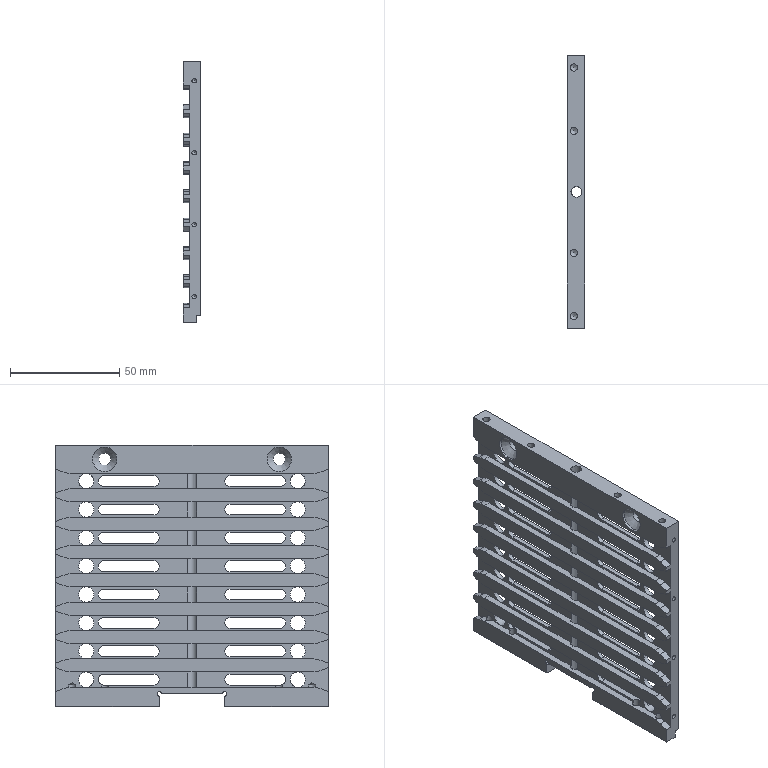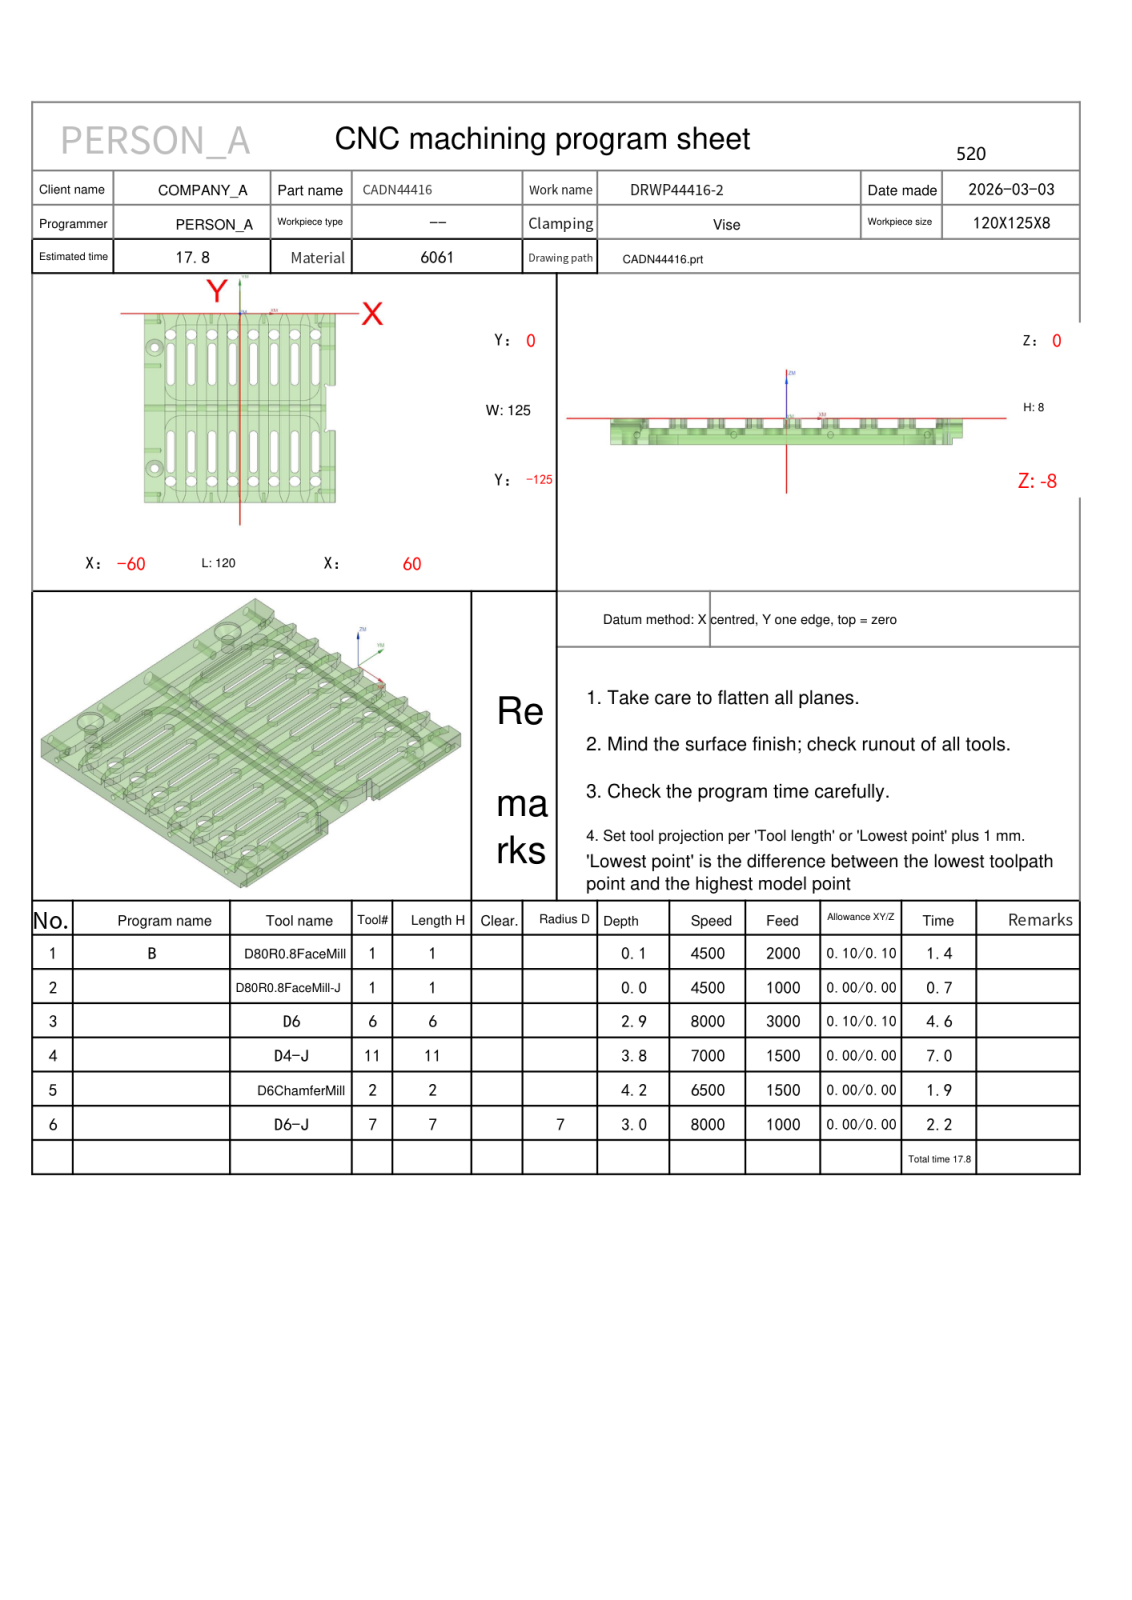NC program | NX | posted by the shop | part box 8 x 125 x 120 mm
Lines 78372 to 79132 of 79132:
N5 T02 M06
(D6ChamferMill  D=6. R=0. H=02 ce=0.00 di=0.00)
G00 G90 G54 X60.21 Y-48.403 M03 S6500
G43 H02 Z50.
M08
Z2.8
G01 Z-1.2 F1500.
X60.059 Y-48.466
X59.8 Y-48.5
X55.732
X55.385 Y-48.47
X55.048 Y-48.379
X54.732 Y-48.232
X54.879 Y-48.548
X54.97 Y-48.885
X55. Y-49.232
Y-75.768
X54.97 Y-76.115
X54.879 Y-76.452
X54.732 Y-76.768
X55.048 Y-76.621
X55.385 Y-76.53
X55.732 Y-76.5
X59.8
X60.059 Y-76.534
X60.21 Y-76.597
Z2.8
G00 Z10.
Y-125.903
Z2.8
G01 Z-1.2
X60.059 Y-125.966
X59.8 Y-126.
X53.002
G02 X52.062 Y-125.342 I0.0 J1.
G01 X50.663 Y-121.499
G02 X50. Y-117.737 I10.337 J3.762
G01 Y-62.5
Y-7.263
G02 X50.663 Y-3.501 I11. J0.0
G01 X52.062 Y.342
G02 X53.002 Y1. I.94 J-.342
G01 X59.8
X60.059 Y.966
X60.21 Y.903
Z2.8
G00 Z10.
X45.227 Y-62.114
Z.172
G01 Z-1.2
G03 X45.027 Y-62.4 I1.532 J-1.286
G01 X44.997 Y-62.446
X45. Y-62.5
Y-117.737
G02 X44.337 Y-121.499 I-11. J0.0
G01 X42.938 Y-125.342
G02 X41.998 Y-126. I-.94 J.342
G01 X40.002
G02 X39.062 Y-125.342 I0.0 J1.
G01 X37.663 Y-121.499
G02 X37. Y-117.737 I10.337 J3.762
G01 Y-7.263
G02 X37.663 Y-3.501 I11. J0.0
G01 X39.062 Y.342
G02 X40.002 Y1. I.94 J-.342
G01 X41.998
G02 X42.938 Y.342 I0.0 J-1.
G01 X44.337 Y-3.501
G02 X45. Y-7.263 I-10.337 J-3.762
G01 Y-62.5
X44.997 Y-62.554
X45.027 Y-62.6
G03 X45.227 Y-62.886 I1.732 J1.
G01 Z.172
G00 Z10.
X32.227 Y-62.114
Z.172
G01 Z-1.2
G03 X32.027 Y-62.4 I1.532 J-1.286
G01 X31.997 Y-62.446
X32. Y-62.5
Y-117.737
G02 X31.337 Y-121.499 I-11. J0.0
G01 X29.938 Y-125.342
G02 X28.998 Y-126. I-.94 J.342
G01 X27.002
G02 X26.062 Y-125.342 I0.0 J1.
G01 X24.663 Y-121.499
G02 X24. Y-117.737 I10.337 J3.762
G01 Y-7.263
G02 X24.663 Y-3.501 I11. J0.0
G01 X26.062 Y.342
G02 X27.002 Y1. I.94 J-.342
G01 X28.998
G02 X29.938 Y.342 I0.0 J-1.
G01 X31.337 Y-3.501
G02 X32. Y-7.263 I-10.337 J-3.762
G01 Y-62.5
X31.997 Y-62.554
X32.027 Y-62.6
G03 X32.227 Y-62.886 I1.732 J1.
G01 Z.172
G00 Z10.
X19.227 Y-62.114
Z.172
G01 Z-1.2
G03 X19.027 Y-62.4 I1.532 J-1.286
G01 X18.997 Y-62.446
X19. Y-62.5
Y-117.737
G02 X18.337 Y-121.499 I-11. J0.0
G01 X16.938 Y-125.342
G02 X15.998 Y-126. I-.94 J.342
G01 X14.002
G02 X13.062 Y-125.342 I0.0 J1.
G01 X11.663 Y-121.499
G02 X11. Y-117.737 I10.337 J3.762
G01 Y-7.263
G02 X11.663 Y-3.501 I11. J0.0
G01 X13.062 Y.342
G02 X14.002 Y1. I.94 J-.342
G01 X15.998
G02 X16.938 Y.342 I0.0 J-1.
G01 X18.337 Y-3.501
G02 X19. Y-7.263 I-10.337 J-3.762
G01 Y-62.5
X18.997 Y-62.554
X19.027 Y-62.6
G03 X19.227 Y-62.886 I1.732 J1.
G01 Z.172
G00 Z10.
X6.227 Y-62.114
Z.172
G01 Z-1.2
G03 X6.027 Y-62.4 I1.532 J-1.286
G01 X5.997 Y-62.446
X6. Y-62.5
Y-117.737
G02 X5.337 Y-121.499 I-11. J0.0
G01 X3.938 Y-125.342
G02 X2.998 Y-126. I-.94 J.342
G01 X1.002
G02 X.062 Y-125.342 I0.0 J1.
G01 X-1.337 Y-121.499
G02 X-2. Y-117.737 I10.337 J3.762
G01 Y-7.263
G02 X-1.337 Y-3.501 I11. J0.0
G01 X.062 Y.342
G02 X1.002 Y1. I.94 J-.342
G01 X2.998
G02 X3.938 Y.342 I0.0 J-1.
G01 X5.337 Y-3.501
G02 X6. Y-7.263 I-10.337 J-3.762
G01 Y-62.5
X5.997 Y-62.554
X6.027 Y-62.6
G03 X6.227 Y-62.886 I1.732 J1.
G01 Z.172
G00 Z10.
X-6.773 Y-62.114
Z.172
G01 Z-1.2
G03 X-6.973 Y-62.4 I1.532 J-1.286
G01 X-7.003 Y-62.446
X-7. Y-62.5
Y-117.737
G02 X-7.663 Y-121.499 I-11. J0.0
G01 X-9.062 Y-125.342
G02 X-10.002 Y-126. I-.94 J.342
G01 X-11.998
G02 X-12.938 Y-125.342 I0.0 J1.
G01 X-14.337 Y-121.499
G02 X-15. Y-117.737 I10.337 J3.762
G01 Y-7.263
G02 X-14.337 Y-3.501 I11. J0.0
G01 X-12.938 Y.342
G02 X-11.998 Y1. I.94 J-.342
G01 X-10.002
G02 X-9.062 Y.342 I0.0 J-1.
G01 X-7.663 Y-3.501
G02 X-7. Y-7.263 I-10.337 J-3.762
G01 Y-62.5
X-7.003 Y-62.554
X-6.973 Y-62.6
G03 X-6.773 Y-62.886 I1.732 J1.
G01 Z.172
G00 Z10.
X-19.773 Y-62.114
Z.172
G01 Z-1.2
G03 X-19.973 Y-62.4 I1.532 J-1.286
G01 X-20.003 Y-62.446
X-20. Y-62.5
Y-117.737
G02 X-20.663 Y-121.499 I-11. J0.0
G01 X-22.062 Y-125.342
G02 X-23.002 Y-126. I-.94 J.342
G01 X-24.998
G02 X-25.938 Y-125.342 I0.0 J1.
G01 X-27.337 Y-121.499
G02 X-28. Y-117.737 I10.337 J3.762
G01 Y-7.263
G02 X-27.337 Y-3.501 I11. J0.0
G01 X-25.938 Y.342
G02 X-24.998 Y1. I.94 J-.342
G01 X-23.002
G02 X-22.062 Y.342 I0.0 J-1.
G01 X-20.663 Y-3.501
G02 X-20. Y-7.263 I-10.337 J-3.762
G01 Y-62.5
X-20.003 Y-62.554
X-19.973 Y-62.6
G03 X-19.773 Y-62.886 I1.732 J1.
G01 Z.172
G00 Z10.
X-32.773 Y-62.114
Z.172
G01 Z-1.2
G03 X-32.973 Y-62.4 I1.532 J-1.286
G01 X-33.003 Y-62.446
X-33. Y-62.5
Y-117.737
G02 X-33.663 Y-121.499 I-11. J0.0
G01 X-35.062 Y-125.342
G02 X-36.002 Y-126. I-.94 J.342
G01 X-37.998
G02 X-38.938 Y-125.342 I0.0 J1.
G01 X-40.337 Y-121.499
G02 X-41. Y-117.737 I10.337 J3.762
G01 Y-7.263
G02 X-40.337 Y-3.501 I11. J0.0
G01 X-38.938 Y.342
G02 X-37.998 Y1. I.94 J-.342
G01 X-36.002
G02 X-35.062 Y.342 I0.0 J-1.
G01 X-33.663 Y-3.501
G02 X-33. Y-7.263 I-10.337 J-3.762
G01 Y-62.5
X-33.003 Y-62.554
X-32.973 Y-62.6
G03 X-32.773 Y-62.886 I1.732 J1.
G01 Z.172
G00 Z10.
X-61.227
Z.172
G01 Z-1.2
G03 X-61.027 Y-62.6 I-1.532 J1.286
G01 X-60.997 Y-62.554
X-61. Y-62.5
Y0.0
G02 X-60. Y1. I1. J0.0
G01 X-49.002
G02 X-48.062 Y.342 I0.0 J-1.
G01 X-46.663 Y-3.501
G02 X-46. Y-7.263 I-10.337 J-3.762
G01 Y-117.737
G02 X-46.663 Y-121.499 I-11. J0.0
G01 X-48.062 Y-125.342
G02 X-49.002 Y-126. I-.94 J.342
G01 X-60.
G02 X-61. Y-125. I0.0 J1.
G01 Y-62.5
X-60.997 Y-62.446
X-61.027 Y-62.4
G03 X-61.227 Y-62.114 I-1.732 J-1.
G01 Z.172
G00 Z10.
X-49.101 Y-102.9
Z.224
G01 Z-1.2
G03 X-48.92 Y-102.602 I-1.613 J1.183
G01 X-48.894 Y-102.554
X-48.9 Y-102.5
G03 X-53.5 Y-97.9 I-4.6 J0.0
X-58.1 Y-102.5 I0.0 J-4.6
X-53.5 Y-107.1 I4.6 J0.0
X-48.9 Y-102.5 I0.0 J4.6
G01 X-48.894 Y-102.446
X-48.92 Y-102.398
G03 X-49.101 Y-102.1 I-1.794 J-.885
G01 Z.224
G00 Z10.
Y-22.9
Z.224
G01 Z-1.2
G03 X-48.92 Y-22.602 I-1.613 J1.183
G01 X-48.894 Y-22.554
X-48.9 Y-22.5
G03 X-53.5 Y-17.9 I-4.6 J0.0
X-58.1 Y-22.5 I0.0 J-4.6
X-53.5 Y-27.1 I4.6 J0.0
X-48.9 Y-22.5 I0.0 J4.6
G01 X-48.894 Y-22.446
X-48.92 Y-22.398
G03 X-49.101 Y-22.1 I-1.794 J-.885
G01 Z.224
G00 Z10.
X-45.98 Y1.068
Z-1.806
G01 Z-4.199
X-45.894 Y1.008
X-45.864 Y1.
X-41.136
X-41.106 Y1.008
X-41.02 Y1.068
Z-1.806
G00 Z3.301
X-32.98
Z-1.806
G01 Z-4.199
X-32.894 Y1.008
X-32.864 Y1.
X-28.136
X-28.106 Y1.008
X-28.02 Y1.068
Z-1.806
G00 Z3.301
X-19.98
Z-1.806
G01 Z-4.199
X-19.894 Y1.008
X-19.864 Y1.
X-15.136
X-15.106 Y1.008
X-15.02 Y1.068
Z-1.806
G00 Z3.301
X-6.98
Z-1.806
G01 Z-4.199
X-6.894 Y1.008
X-6.864 Y1.
X-2.136
X-2.106 Y1.008
X-2.02 Y1.068
Z-1.806
G00 Z3.301
X6.02
Z-1.806
G01 Z-4.199
X6.106 Y1.008
X6.136 Y1.
X10.864
X10.894 Y1.008
X10.98 Y1.068
Z-1.806
G00 Z3.301
X19.02
Z-1.806
G01 Z-4.199
X19.106 Y1.008
X19.136 Y1.
X23.864
X23.894 Y1.008
X23.98 Y1.068
Z-1.806
G00 Z3.301
X32.02
Z-1.806
G01 Z-4.199
X32.106 Y1.008
X32.136 Y1.
X36.864
X36.894 Y1.008
X36.98 Y1.068
Z-1.806
G00 Z3.301
X45.02
Z-1.806
G01 Z-4.199
X45.106 Y1.008
X45.136 Y1.
X49.864
X49.894 Y1.008
X49.98 Y1.068
Z-1.806
G00 Z10.
Y-126.068
Z-1.806
G01 Z-4.199
X49.894 Y-126.008
X49.864 Y-126.
X45.136
X45.106 Y-126.008
X45.02 Y-126.068
Z-1.806
G00 Z3.301
X36.98
Z-1.806
G01 Z-4.199
X36.894 Y-126.008
X36.864 Y-126.
X32.136
X32.106 Y-126.008
X32.02 Y-126.068
Z-1.806
G00 Z3.301
X23.98
Z-1.806
G01 Z-4.199
X23.894 Y-126.008
X23.864 Y-126.
X19.136
X19.106 Y-126.008
X19.02 Y-126.068
Z-1.806
G00 Z3.301
X10.98
Z-1.806
G01 Z-4.199
X10.894 Y-126.008
X10.864 Y-126.
X6.136
X6.106 Y-126.008
X6.02 Y-126.068
Z-1.806
G00 Z3.301
X-2.02
Z-1.806
G01 Z-4.199
X-2.106 Y-126.008
X-2.136 Y-126.
X-6.864
X-6.894 Y-126.008
X-6.98 Y-126.068
Z-1.806
G00 Z3.301
X-15.02
Z-1.806
G01 Z-4.199
X-15.106 Y-126.008
X-15.136 Y-126.
X-19.864
X-19.894 Y-126.008
X-19.98 Y-126.068
Z-1.806
G00 Z3.301
X-28.02
Z-1.806
G01 Z-4.199
X-28.106 Y-126.008
X-28.136 Y-126.
X-32.864
X-32.894 Y-126.008
X-32.98 Y-126.068
Z-1.806
G00 Z3.301
X-41.02
Z-1.806
G01 Z-4.199
X-41.106 Y-126.008
X-41.136 Y-126.
X-45.864
X-45.894 Y-126.008
X-45.98 Y-126.068
Z-1.806
G00 Z50.
G00 G90 X61.9 Y-73.537 M03 S6500
Z50.
Z.6
G01 Z-.9 F1500.
G03 X60.7 Y-74.737 I0.0 J-1.2
G01 Y-127.763
G03 X61.9 Y-128.963 I1.2 J0.0
G01 Z.6
G00 Z50.
Y3.963
Z.6
G01 Z-.9
G03 X60.7 Y2.763 I0.0 J-1.2
G01 Y-50.263
G03 X61.9 Y-51.463 I1.2 J0.0
G01 Z.6
G00 Z50.
G91 G28 Z0.0
M05
M09
G91 G28 Z0.0
M01
N6 T07 M06
(D6-J  D=6. R=0. H=07 ce=0.00 di=0.00)
G00 G90 G54 X49.562 Y-127.228 M03 S8000
G43 H07 Z6.8
M08
Z-2.
G01 Z-3. F1000.
G41 D07
X49.74 Y-127.138
G03 X50.237 Y-126.334 I-.403 J.805
X50.183 Y-126.026 I-.9 J0.0
G01 X48.784 Y-122.183
G02 X48. Y-117.737 I12.216 J4.446
G01 Y-7.263
G02 X48.784 Y-2.817 I13. J0.0
G01 X50.183 Y1.026
G03 X50.237 Y1.334 I-.846 J.308
X49.74 Y2.138 I-.9 J0.0
G01 G40 X49.562 Y2.228
Z-2.
G00 Z6.8
X36.562 Y-127.228
Z-2.
G01 Z-3.
G41 D07
X36.74 Y-127.138
G03 X37.237 Y-126.334 I-.403 J.805
X37.183 Y-126.026 I-.9 J0.0
G01 X35.784 Y-122.183
G02 X35. Y-117.737 I12.216 J4.446
G01 Y-7.263
G02 X35.784 Y-2.817 I13. J0.0
G01 X37.183 Y1.026
G03 X37.237 Y1.334 I-.846 J.308
X36.74 Y2.138 I-.9 J0.0
G01 G40 X36.562 Y2.228
Z-2.
G00 Z6.8
X45.438
Z-2.
G01 Z-3.
G41 D07
X45.26 Y2.138
G03 X44.763 Y1.334 I.403 J-.805
X44.817 Y1.026 I.9 J0.0
G01 X46.216 Y-2.817
G02 X47. Y-7.263 I-12.216 J-4.446
G01 Y-117.737
G02 X46.216 Y-122.183 I-13. J0.0
G01 X44.817 Y-126.026
G03 X44.763 Y-126.334 I.846 J-.308
X45.26 Y-127.138 I.9 J0.0
G01 G40 X45.438 Y-127.228
Z-2.
G00 Z6.8
X23.562
Z-2.
G01 Z-3.
G41 D07
X23.74 Y-127.138
G03 X24.237 Y-126.334 I-.403 J.805
X24.183 Y-126.026 I-.9 J0.0
G01 X22.784 Y-122.183
G02 X22. Y-117.737 I12.216 J4.446
G01 Y-7.263
G02 X22.784 Y-2.817 I13. J0.0
G01 X24.183 Y1.026
G03 X24.237 Y1.334 I-.846 J.308
X23.74 Y2.138 I-.9 J0.0
G01 G40 X23.562 Y2.228
Z-2.
G00 Z6.8
X32.438
Z-2.
G01 Z-3.
G41 D07
X32.26 Y2.138
G03 X31.763 Y1.334 I.403 J-.805
X31.817 Y1.026 I.9 J0.0
G01 X33.216 Y-2.817
G02 X34. Y-7.263 I-12.216 J-4.446
G01 Y-117.737
G02 X33.216 Y-122.183 I-13. J0.0
G01 X31.817 Y-126.026
G03 X31.763 Y-126.334 I.846 J-.308
X32.26 Y-127.138 I.9 J0.0
G01 G40 X32.438 Y-127.228
Z-2.
G00 Z6.8
X10.562
Z-2.
G01 Z-3.
G41 D07
X10.74 Y-127.138
G03 X11.237 Y-126.334 I-.403 J.805
X11.183 Y-126.026 I-.9 J0.0
G01 X9.784 Y-122.183
G02 X9. Y-117.737 I12.216 J4.446
G01 Y-7.263
G02 X9.784 Y-2.817 I13. J0.0
G01 X11.183 Y1.026
G03 X11.237 Y1.334 I-.846 J.308
X10.74 Y2.138 I-.9 J0.0
G01 G40 X10.562 Y2.228
Z-2.
G00 Z6.8
X19.438
Z-2.
G01 Z-3.
G41 D07
X19.26 Y2.138
G03 X18.763 Y1.334 I.403 J-.805
X18.817 Y1.026 I.9 J0.0
G01 X20.216 Y-2.817
G02 X21. Y-7.263 I-12.216 J-4.446
G01 Y-117.737
G02 X20.216 Y-122.183 I-13. J0.0
G01 X18.817 Y-126.026
G03 X18.763 Y-126.334 I.846 J-.308
X19.26 Y-127.138 I.9 J0.0
G01 G40 X19.438 Y-127.228
Z-2.
G00 Z6.8
X-2.438
Z-2.
G01 Z-3.
G41 D07
X-2.26 Y-127.138
G03 X-1.763 Y-126.334 I-.403 J.805
X-1.817 Y-126.026 I-.9 J0.0
G01 X-3.216 Y-122.183
G02 X-4. Y-117.737 I12.216 J4.446
G01 Y-7.263
G02 X-3.216 Y-2.817 I13. J0.0
G01 X-1.817 Y1.026
G03 X-1.763 Y1.334 I-.846 J.308
X-2.26 Y2.138 I-.9 J0.0
G01 G40 X-2.438 Y2.228
Z-2.
G00 Z6.8
X6.438
Z-2.
G01 Z-3.
G41 D07
X6.26 Y2.138
G03 X5.763 Y1.334 I.403 J-.805
X5.817 Y1.026 I.9 J0.0
G01 X7.216 Y-2.817
G02 X8. Y-7.263 I-12.216 J-4.446
G01 Y-117.737
G02 X7.216 Y-122.183 I-13. J0.0
G01 X5.817 Y-126.026
G03 X5.763 Y-126.334 I.846 J-.308
X6.26 Y-127.138 I.9 J0.0
G01 G40 X6.438 Y-127.228
Z-2.
G00 Z6.8
X-15.438
Z-2.
G01 Z-3.
G41 D07
X-15.26 Y-127.138
G03 X-14.763 Y-126.334 I-.403 J.805
X-14.817 Y-126.026 I-.9 J0.0
G01 X-16.216 Y-122.183
G02 X-17. Y-117.737 I12.216 J4.446
G01 Y-7.263
G02 X-16.216 Y-2.817 I13. J0.0
G01 X-14.817 Y1.026
G03 X-14.763 Y1.334 I-.846 J.308
X-15.26 Y2.138 I-.9 J0.0
G01 G40 X-15.438 Y2.228
Z-2.
G00 Z6.8
X-6.562
Z-2.
G01 Z-3.
G41 D07
X-6.74 Y2.138
G03 X-7.237 Y1.334 I.403 J-.805
X-7.183 Y1.026 I.9 J0.0
G01 X-5.784 Y-2.817
G02 X-5. Y-7.263 I-12.216 J-4.446
G01 Y-117.737
G02 X-5.784 Y-122.183 I-13. J0.0
G01 X-7.183 Y-126.026
G03 X-7.237 Y-126.334 I.846 J-.308
X-6.74 Y-127.138 I.9 J0.0
G01 G40 X-6.562 Y-127.228
Z-2.
G00 Z6.8
X-28.438
Z-2.
G01 Z-3.
G41 D07
X-28.26 Y-127.138
G03 X-27.763 Y-126.334 I-.403 J.805
X-27.817 Y-126.026 I-.9 J0.0
G01 X-29.216 Y-122.183
G02 X-30. Y-117.737 I12.216 J4.446
G01 Y-7.263
G02 X-29.216 Y-2.817 I13. J0.0
G01 X-27.817 Y1.026
G03 X-27.763 Y1.334 I-.846 J.308
X-28.26 Y2.138 I-.9 J0.0
G01 G40 X-28.438 Y2.228
Z-2.
G00 Z6.8
X-19.562
Z-2.
G01 Z-3.
G41 D07
X-19.74 Y2.138
G03 X-20.237 Y1.334 I.403 J-.805
X-20.183 Y1.026 I.9 J0.0
G01 X-18.784 Y-2.817
G02 X-18. Y-7.263 I-12.216 J-4.446
G01 Y-117.737
G02 X-18.784 Y-122.183 I-13. J0.0
G01 X-20.183 Y-126.026
G03 X-20.237 Y-126.334 I.846 J-.308
X-19.74 Y-127.138 I.9 J0.0
G01 G40 X-19.562 Y-127.228
Z-2.
G00 Z6.8
X-41.438
Z-2.
G01 Z-3.
G41 D07
X-41.26 Y-127.138
G03 X-40.763 Y-126.334 I-.403 J.805
X-40.817 Y-126.026 I-.9 J0.0
G01 X-42.216 Y-122.183
G02 X-43. Y-117.737 I12.216 J4.446
G01 Y-7.263
G02 X-42.216 Y-2.817 I13. J0.0
G01 X-40.817 Y1.026
G03 X-40.763 Y1.334 I-.846 J.308
X-41.26 Y2.138 I-.9 J0.0
G01 G40 X-41.438 Y2.228
Z-2.
G00 Z6.8
X-32.562
Z-2.
G01 Z-3.
G41 D07
X-32.74 Y2.138
G03 X-33.237 Y1.334 I.403 J-.805
X-33.183 Y1.026 I.9 J0.0
G01 X-31.784 Y-2.817
G02 X-31. Y-7.263 I-12.216 J-4.446
G01 Y-117.737
G02 X-31.784 Y-122.183 I-13. J0.0
G01 X-33.183 Y-126.026
G03 X-33.237 Y-126.334 I.846 J-.308
X-32.74 Y-127.138 I.9 J0.0
G01 G40 X-32.562 Y-127.228
Z-2.
G00 Z6.8
X-45.562 Y2.228
Z-2.
G01 Z-3.
G41 D07
X-45.74 Y2.138
G03 X-46.237 Y1.334 I.403 J-.805
X-46.183 Y1.026 I.9 J0.0
G01 X-44.784 Y-2.817
G02 X-44. Y-7.263 I-12.216 J-4.446
G01 Y-117.737
G02 X-44.784 Y-122.183 I-13. J0.0
G01 X-46.183 Y-126.026
G03 X-46.237 Y-126.334 I.846 J-.308
X-45.74 Y-127.138 I.9 J0.0
G01 G40 X-45.562 Y-127.228
Z-2.
G00 Z6.8
M05
M09
G91 G28 Z0.0
G91 G28 Y0.0
M30
%